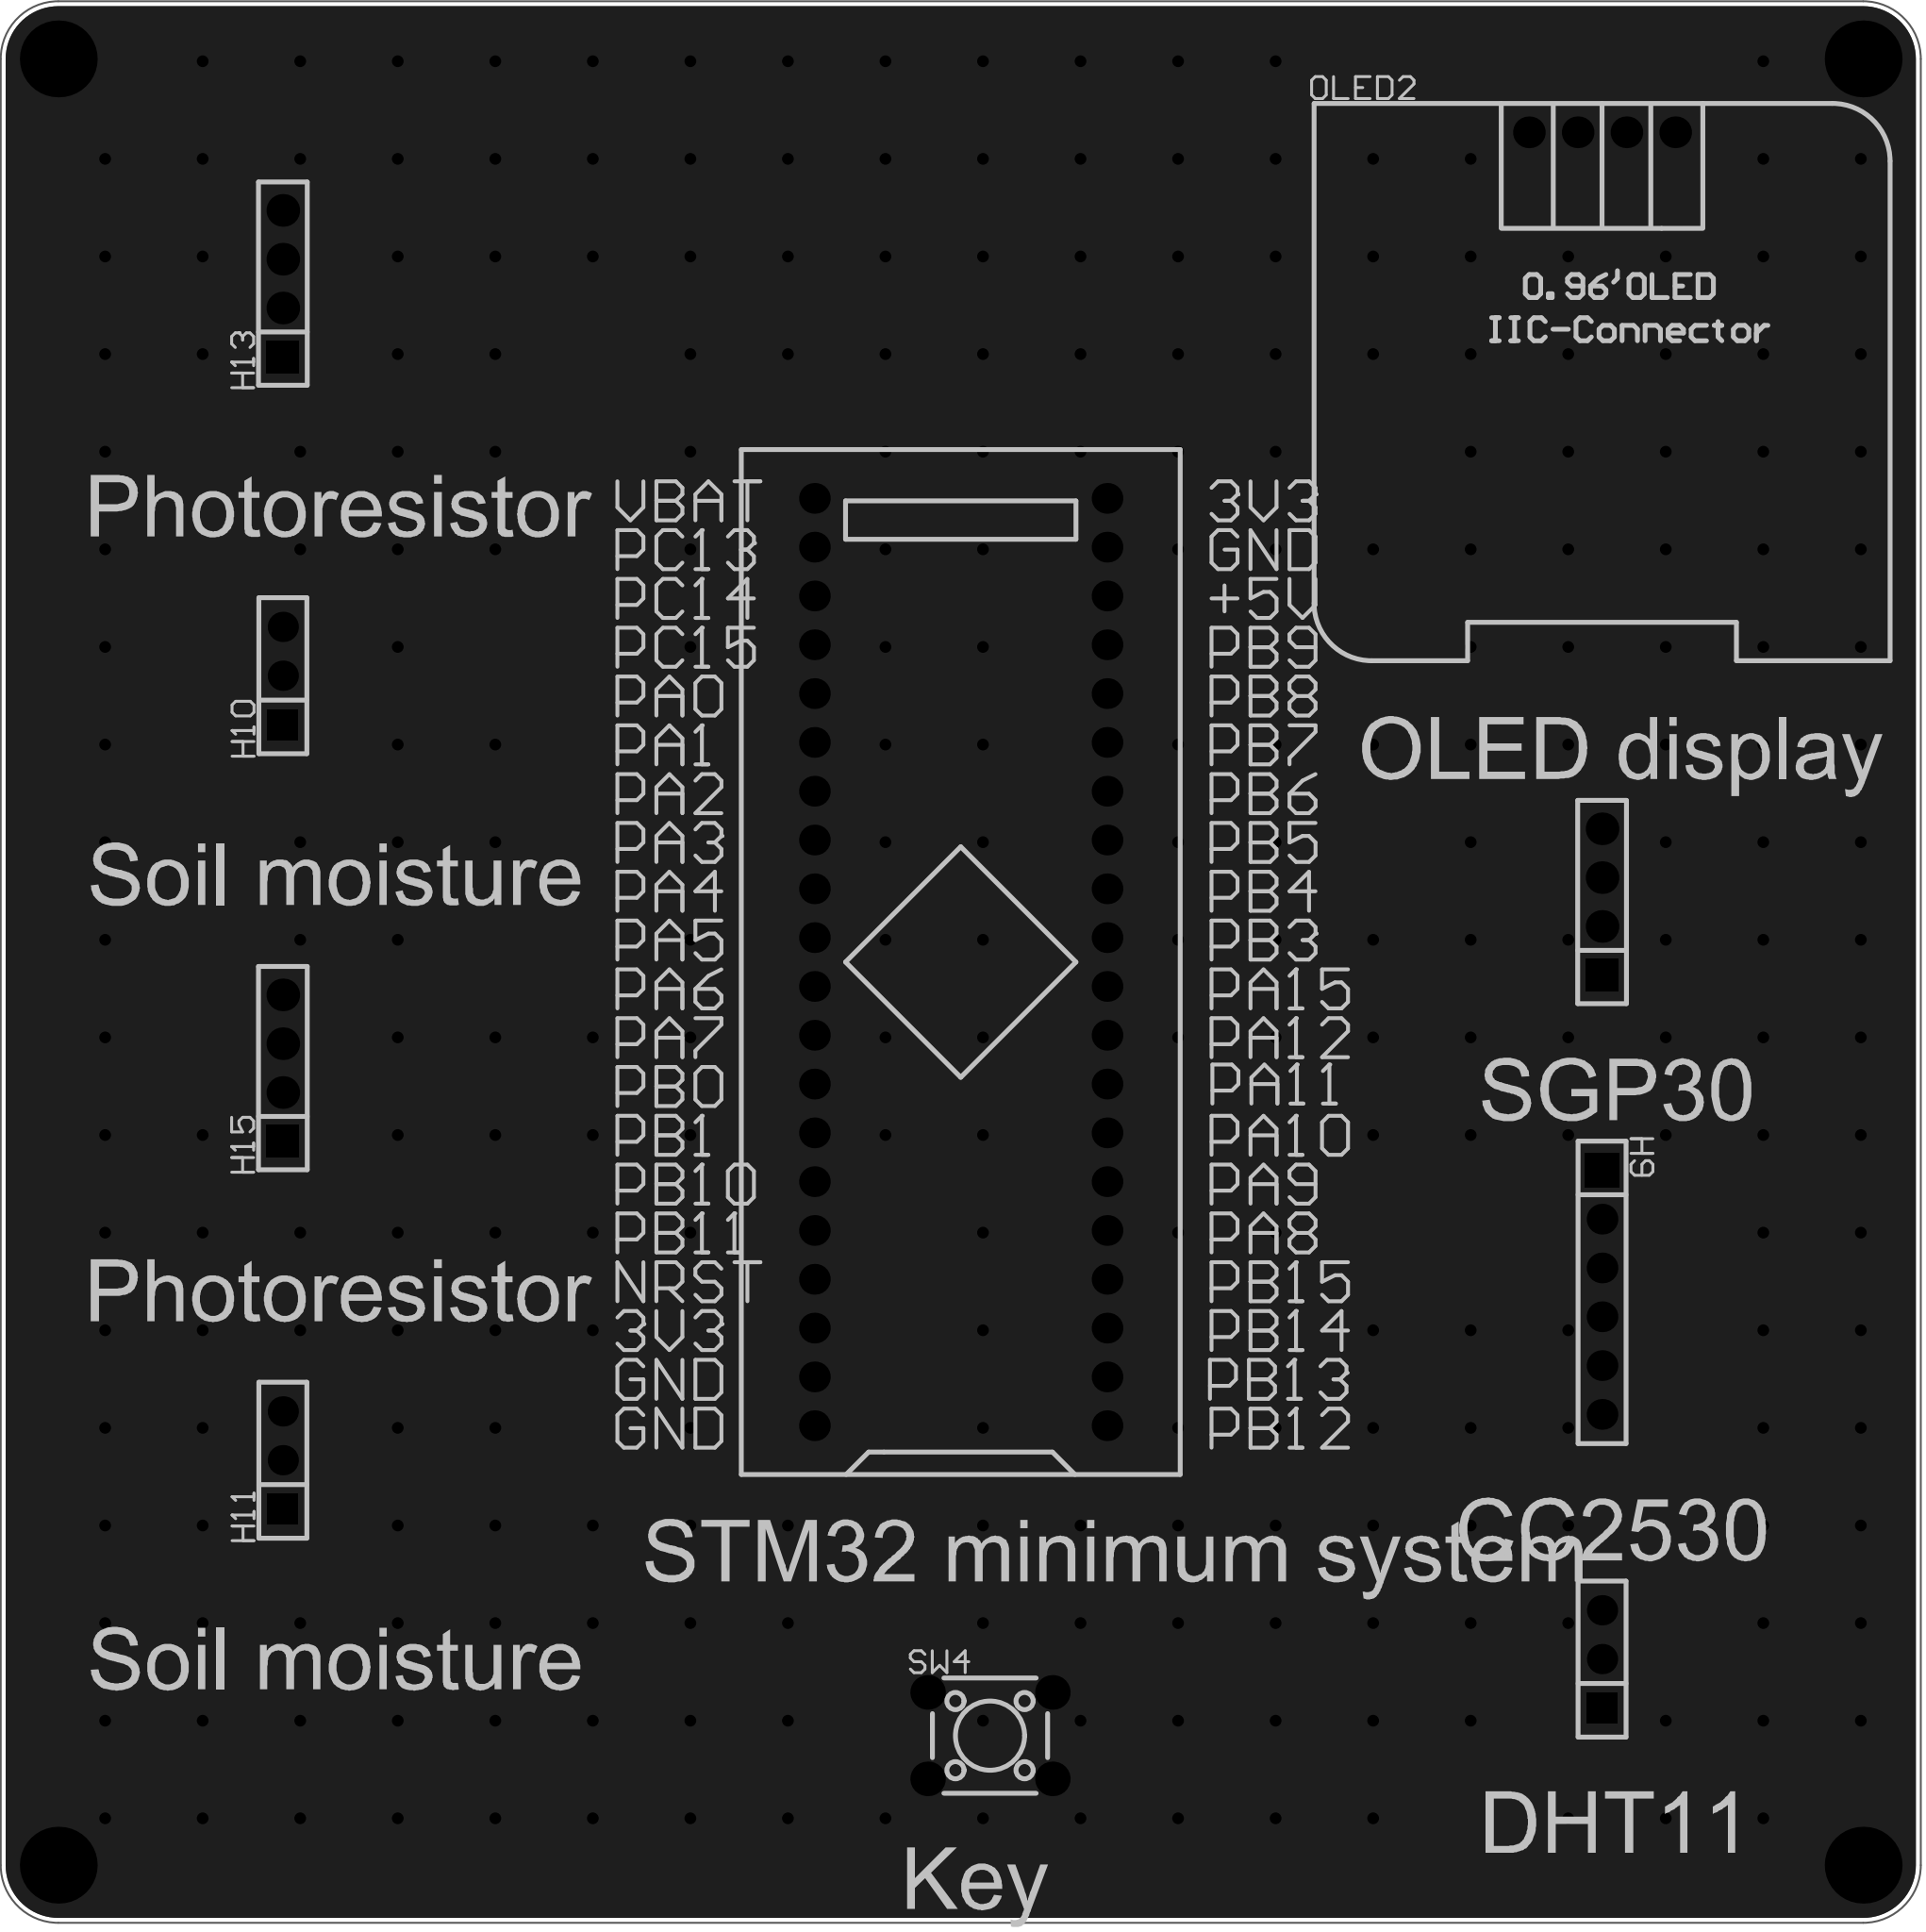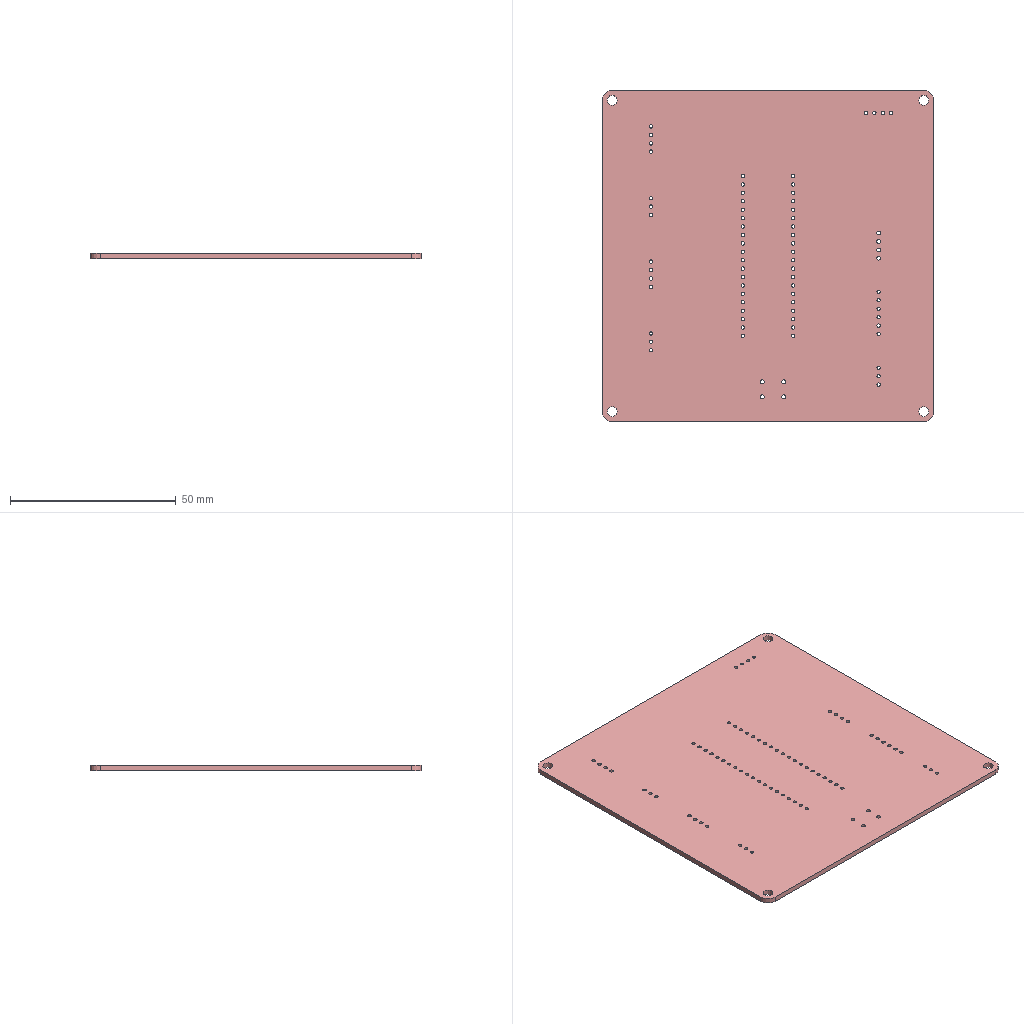Circuit board layout | Altium Designer | box 100 x 100 x 1.6 mm
Layer stack:
# Altium Designer layer stack of  (unit mm; dielectric type: 0 none, 1 core, 2 prepreg, 3 surface material)
index,name,kind,layer,copper_thickness_mm,dielectric_type,dielectric_thickness_mm,dielectric_material,dielectric_constant
0,Top Paste Mask Layer,other,,,,,,
1,Top Silkscreen Layer,other,,,,,,
2,Top Solder Mask Layer,dielectric,,,3,0.01,,3.3
3,Top Layer,copper,Top Layer,0.035,,,,
4,Dielectric1,dielectric,,,3,1.51,FR4,4.5
5,Bottom Layer,copper,Bottom Layer,0.035,,,,
6,Bottom Solder Mask Layer,dielectric,,,3,0.01,,3.3
7,Bottom Silkscreen Layer,other,,,,,,
8,Bottom Paste Mask Layer,other,,,,,,
# drill layer pairs: low layer,high layer
drill_pair,Top Layer,Bottom Layer
Part placement:
Designator,Comment,Layer,Footprint,Center-X(mm),Center-Y(mm),Rotation
U1,STM32F103C8T6-Card,TopLayer,CONN-TH_L53.3-W22.9_STM32F103C8T6-CARD,141.351,130.937,90
SW4,,TopLayer,SW-TH_4P-L6.0-W6.0-P4.50-LS6.5,142.875,90.678,0
H3,,TopLayer,HDR-TH_3P-P2.54-V-F,174.752,94.662,90
H4,,TopLayer,HDR-TH_4P-P2.54-V-F,174.752,134.06,90
OLED2,,TopLayer,0.96OLED_4P,174.752,174.117,0
H9,,TopLayer,HDR-TH_6P-P2.54-V-F,174.752,113.746,270
H10,,TopLayer,HDR-TH_3P-P2.54-V-F,106.045,145.838,90
H11,,TopLayer,HDR-TH_3P-P2.54-V-F,106.045,105.012,90
H13,,TopLayer,HDR-TH_4P-P2.54-V-F,106.045,166.243,90
H15,,TopLayer,HDR-TH_4P-P2.54-V-F,106.045,125.417,90
Pad and via stacks:
# Altium Designer via and pad stacks of  (unit mm). Each distinct definition once, with the count of objects using it.
# via: kind,start_layer,end_layer,hole_mm,diameter_mm,mode(0 simple;1 top-mid-bottom;2 full stack),diameter_per_layer,count,example_net
# pad: kind,layer,hole_mm,hole_type(0 round;1 square;2 slot),plating,top_size,top_shape(1 round;2 rect;3 octagon;9 rounded rect),mid_size,bottom_size,mode,footprint,size_per_layer,count,example
pad,Multi-Layer,3,0,plated,4x4,1,4x4,4x4,0,,,4,1
pad,Multi-Layer,1,0,plated,1.6x1.6,1,1.6x1.6,1.6x1.6,0,CONN-TH_L53.3-W22.9_STM32F103C8T6-CARD,,40,U1.1
pad,Multi-Layer,1.2,0,plated,1.8x1.8,1,1.8x1.8,1.8x1.8,0,SW-TH_4P-L6.0-W6.0-P4.50-LS6.5,,4,SW4.1
pad,Multi-Layer,1.02,0,plated,1.575x1.575,1,1.575x1.575,1.575x1.575,0,HDR-TH_3P-P2.54-V-F,,6,H3.3
pad,Multi-Layer,1.02,0,plated,1.575x1.575,2,1.575x1.575,1.575x1.575,0,HDR-TH_3P-P2.54-V-F,,3,H3.1
pad,Multi-Layer,1.1,0,plated,1.7x1.7,2,1.7x1.7,1.7x1.7,0,HDR-TH_4P-P2.54-V-F,,3,H4.1
pad,Multi-Layer,1.1,0,plated,1.7x1.7,1,1.7x1.7,1.7x1.7,0,HDR-TH_4P-P2.54-V-F,,9,H4.2
pad,Multi-Layer,1,0,plated,1.65x1.65,1,1.65x1.65,1.65x1.65,0,0.96OLED_4P,,4,OLED2.4
pad,Multi-Layer,1.02,0,plated,1.6x1.6,1,1.6x1.6,1.6x1.6,0,HDR-TH_6P-P2.54-V-F,,5,H9.6
pad,Multi-Layer,1.02,0,plated,1.8x1.8,2,1.8x1.8,1.8x1.8,0,HDR-TH_6P-P2.54-V-F,,1,H9.1
via,Top Layer,Bottom Layer,0.3048,0.61,0,,277,GND
Copper pours:
name,layer,net,type(0 solid;1 hatched;2 none)
Bottom Layer-GND,Bottom Layer,GND,0
Top Layer-GND,Top Layer,GND,0
Design rules, without the lines most boards share:
# Altium Designer design rules of  (exported by Altium Designer, unit mm)
# columns: name | kind | enabled | priority | scope1 | scope2 | descriptor | typed fields (field=value)
Copper_copperRegion_copperThickness1oz | 0 | disabled | 4 | All | All | Clearance Constraint (Gap=5.984mil) (Disabled)(All),(All) | gap=0.152
Copper_copperRegion_copperThickness1oz_1 | 63 | disabled | 4 | All | All | Board Clearance Constraint (Gap=0mil) (Disabled)(All) |
Copper_copperRegion_Copper_copperRegion | 0 | disabled | 5 | All | All | Clearance Constraint (Gap=5.984mil) (Disabled)(All),(All) | gap=0.152
Copper_copperRegion_Copper_copperRegion_1 | 63 | disabled | 5 | All | All | Board Clearance Constraint (Gap=0mil) (Disabled)(All) |
copperThickness1oz | 0 | enabled | 6 | All | All | Clearance Constraint (Gap=5.984mil) (All),(All) | gap=0.152
copperThickness1oz_1 | 63 | enabled | 6 | All | All | Board Clearance Constraint (Gap=0mil) (All) |
copperRegion_copperThickness1oz | 20 | disabled | 1 | All | All | Polygon Connect Rule(Relief Connect )(Conductor Width=10mil) (Relief Angle=90 Angle) (Entries=4) (Air Gap Width=10mil) (Disabled)(All),(All) | connect_style(0=relief,1=direct,2=none)=0 relief_conductor_width=0.254 relief_entries=4
copperRegion_Copper_copperRegion | 20 | disabled | 2 | All | All | Polygon Connect Rule(Relief Connect )(Conductor Width=10mil) (Relief Angle=90 Angle) (Entries=4) (Air Gap Width=10mil) (Disabled)(All),(All) | connect_style(0=relief,1=direct,2=none)=0 relief_conductor_width=0.254 relief_entries=4
copperRegion | 20 | enabled | 3 | All | All | Polygon Connect Rule(Relief Connect )(Conductor Width=10mil) (Relief Angle=90 Angle) (Entries=4) (Air Gap Width=10mil) (All),(All) | connect_style(0=relief,1=direct,2=none)=0 relief_conductor_width=0.254 relief_entries=4